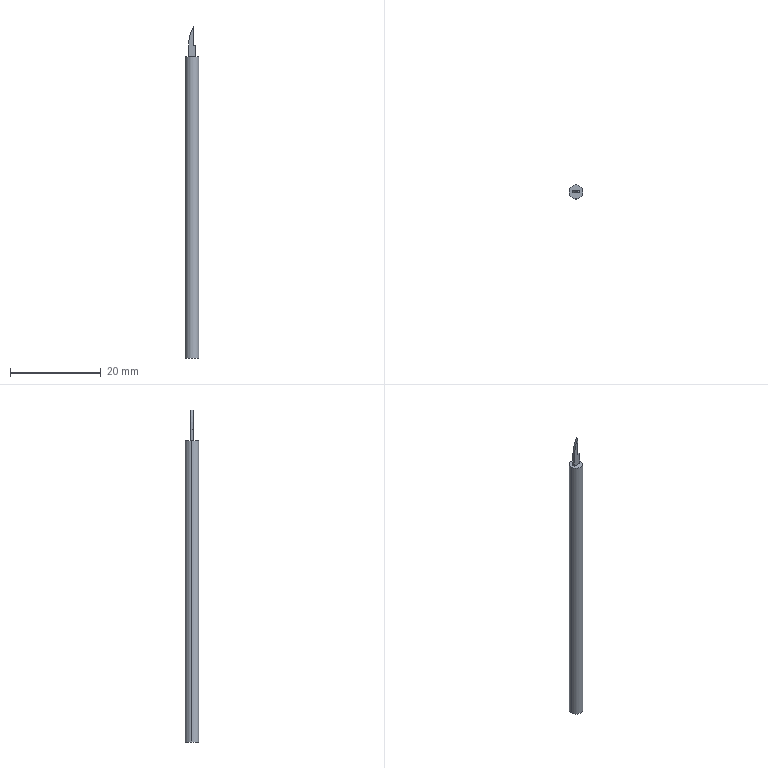Part | SolidWorks | features ICE 2, Extrusion 1 | 1 solid | 11 faces | box 3 x 3 x 73.338 mm | volume 473.804 mm3 | plane 8 | cylinder 3 | commonest cylinder face diameters 3 x2 16.855 x1
STEP:
#1=CARTESIAN_POINT('',(1.5,0.,-46.));
#2=VERTEX_POINT('',#1);
#3=CARTESIAN_POINT('',(-1.5,0.,-46.));
#4=VERTEX_POINT('',#3);
#5=CARTESIAN_POINT('',(0.,0.,-46.));
#6=DIRECTION('',(0.,0.,1.));
#7=DIRECTION('',(1.,0.,0.));
#8=AXIS2_PLACEMENT_3D('',#5,#6,#7);
#9=CIRCLE('',#8,1.5);
#10=EDGE_CURVE('',#2,#4,#9,.T.);
#11=ORIENTED_EDGE('',*,*,#10,.T.);
#12=CARTESIAN_POINT('',(-1.5,0.,20.5));
#13=VERTEX_POINT('',#12);
#14=CARTESIAN_POINT('',(-1.5,0.,-46.));
#15=DIRECTION('',(0.,0.,1.));
#16=VECTOR('',#15,1000.);
#17=LINE('',#14,#16);
#18=EDGE_CURVE('',#4,#13,#17,.T.);
#19=ORIENTED_EDGE('',*,*,#18,.T.);
#20=CARTESIAN_POINT('',(1.5,0.,20.5));
#21=VERTEX_POINT('',#20);
#22=CARTESIAN_POINT('',(0.,0.,20.5));
#23=DIRECTION('',(0.,0.,1.));
#24=DIRECTION('',(1.,0.,0.));
#25=AXIS2_PLACEMENT_3D('',#22,#23,#24);
#26=CIRCLE('',#25,1.5);
#27=EDGE_CURVE('',#21,#13,#26,.T.);
#28=ORIENTED_EDGE('',*,*,#27,.F.);
#29=CARTESIAN_POINT('',(1.5,0.,-46.));
#30=DIRECTION('',(0.,0.,1.));
#31=VECTOR('',#30,1000.);
#32=LINE('',#29,#31);
#33=EDGE_CURVE('',#2,#21,#32,.T.);
#34=ORIENTED_EDGE('',*,*,#33,.F.);
#35=EDGE_LOOP('',(#11,#19,#28,#34));
#36=FACE_OUTER_BOUND('',#35,.T.);
#37=CARTESIAN_POINT('',(0.,0.,-46.));
#38=DIRECTION('',(0.,0.,1.));
#39=DIRECTION('',(1.,0.,0.));
#40=AXIS2_PLACEMENT_3D('',#37,#38,#39);
#41=CYLINDRICAL_SURFACE('',#40,1.5);
#42=ADVANCED_FACE('',(#36),#41,.T.);
#43=ORIENTED_EDGE('',*,*,#27,.T.);
#44=CARTESIAN_POINT('',(0.,0.,20.5));
#45=DIRECTION('',(0.,0.,1.));
#46=DIRECTION('',(1.,0.,0.));
#47=AXIS2_PLACEMENT_3D('',#44,#45,#46);
#48=CIRCLE('',#47,1.5);
#49=EDGE_CURVE('',#13,#21,#48,.T.);
#50=ORIENTED_EDGE('',*,*,#49,.T.);
#51=EDGE_LOOP('',(#43,#50));
#52=FACE_OUTER_BOUND('',#51,.T.);
#53=CARTESIAN_POINT('',(0.8739,0.25,20.5));
#54=VERTEX_POINT('',#53);
#55=CARTESIAN_POINT('',(0.8739,-0.25,20.5));
#56=VERTEX_POINT('',#55);
#57=CARTESIAN_POINT('',(0.8739,0.25,20.5));
#58=DIRECTION('',(0.,-1.,0.));
#59=VECTOR('',#58,1000.);
#60=LINE('',#57,#59);
#61=EDGE_CURVE('',#54,#56,#60,.T.);
#62=ORIENTED_EDGE('',*,*,#61,.T.);
#63=CARTESIAN_POINT('',(-0.7579,-0.25,20.5));
#64=VERTEX_POINT('',#63);
#65=CARTESIAN_POINT('',(0.8739,-0.25,20.5));
#66=DIRECTION('',(-1.,0.,0.));
#67=VECTOR('',#66,1000.);
#68=LINE('',#65,#67);
#69=EDGE_CURVE('',#56,#64,#68,.T.);
#70=ORIENTED_EDGE('',*,*,#69,.T.);
#71=CARTESIAN_POINT('',(-0.7579,0.25,20.5));
#72=VERTEX_POINT('',#71);
#73=CARTESIAN_POINT('',(-0.7579,0.25,20.5));
#74=DIRECTION('',(0.,-1.,0.));
#75=VECTOR('',#74,1000.);
#76=LINE('',#73,#75);
#77=EDGE_CURVE('',#72,#64,#76,.T.);
#78=ORIENTED_EDGE('',*,*,#77,.F.);
#79=CARTESIAN_POINT('',(0.8739,0.25,20.5));
#80=DIRECTION('',(-1.,0.,0.));
#81=VECTOR('',#80,1000.);
#82=LINE('',#79,#81);
#83=EDGE_CURVE('',#54,#72,#82,.T.);
#84=ORIENTED_EDGE('',*,*,#83,.F.);
#85=EDGE_LOOP('',(#62,#70,#78,#84));
#86=FACE_BOUND('',#85,.T.);
#87=CARTESIAN_POINT('',(0.,0.,20.5));
#88=DIRECTION('',(0.,0.,1.));
#89=DIRECTION('',(1.,0.,0.));
#90=AXIS2_PLACEMENT_3D('',#87,#88,#89);
#91=PLANE('',#90);
#92=ADVANCED_FACE('',(#52,#86),#91,.T.);
#93=ORIENTED_EDGE('',*,*,#18,.F.);
#94=CARTESIAN_POINT('',(0.,0.,-46.));
#95=DIRECTION('',(0.,0.,1.));
#96=DIRECTION('',(1.,0.,0.));
#97=AXIS2_PLACEMENT_3D('',#94,#95,#96);
#98=CIRCLE('',#97,1.5);
#99=EDGE_CURVE('',#4,#2,#98,.T.);
#100=ORIENTED_EDGE('',*,*,#99,.T.);
#101=ORIENTED_EDGE('',*,*,#33,.T.);
#102=ORIENTED_EDGE('',*,*,#49,.F.);
#103=EDGE_LOOP('',(#93,#100,#101,#102));
#104=FACE_OUTER_BOUND('',#103,.T.);
#105=CARTESIAN_POINT('',(0.,0.,-46.));
#106=DIRECTION('',(0.,0.,1.));
#107=DIRECTION('',(1.,0.,0.));
#108=AXIS2_PLACEMENT_3D('',#105,#106,#107);
#109=CYLINDRICAL_SURFACE('',#108,1.5);
#110=ADVANCED_FACE('',(#104),#109,.T.);
#111=ORIENTED_EDGE('',*,*,#10,.F.);
#112=ORIENTED_EDGE('',*,*,#99,.F.);
#113=EDGE_LOOP('',(#111,#112));
#114=FACE_OUTER_BOUND('',#113,.T.);
#115=CARTESIAN_POINT('',(0.,0.,-46.));
#116=DIRECTION('',(0.,0.,1.));
#117=DIRECTION('',(1.,0.,0.));
#118=AXIS2_PLACEMENT_3D('',#115,#116,#117);
#119=PLANE('',#118);
#120=ADVANCED_FACE('',(#114),#119,.F.);
#121=CARTESIAN_POINT('',(0.8739,-0.25,23.139));
#122=VERTEX_POINT('',#121);
#123=CARTESIAN_POINT('',(0.8739,-0.25,23.139));
#124=DIRECTION('',(0.,0.,-1.));
#125=VECTOR('',#124,1000.);
#126=LINE('',#123,#125);
#127=EDGE_CURVE('',#122,#56,#126,.T.);
#128=ORIENTED_EDGE('',*,*,#127,.T.);
#129=ORIENTED_EDGE('',*,*,#61,.F.);
#130=CARTESIAN_POINT('',(0.8739,0.25,23.139));
#131=VERTEX_POINT('',#130);
#132=CARTESIAN_POINT('',(0.8739,0.25,23.139));
#133=DIRECTION('',(0.,0.,-1.));
#134=VECTOR('',#133,1000.);
#135=LINE('',#132,#134);
#136=EDGE_CURVE('',#131,#54,#135,.T.);
#137=ORIENTED_EDGE('',*,*,#136,.F.);
#138=CARTESIAN_POINT('',(0.8739,0.25,23.139));
#139=DIRECTION('',(0.,-1.,0.));
#140=VECTOR('',#139,1000.);
#141=LINE('',#138,#140);
#142=EDGE_CURVE('',#131,#122,#141,.T.);
#143=ORIENTED_EDGE('',*,*,#142,.T.);
#144=EDGE_LOOP('',(#128,#129,#137,#143));
#145=FACE_OUTER_BOUND('',#144,.T.);
#146=CARTESIAN_POINT('',(0.8739,0.25,23.139));
#147=DIRECTION('',(-1.,0.,0.));
#148=DIRECTION('',(0.,-1.,0.));
#149=AXIS2_PLACEMENT_3D('',#146,#147,#148);
#150=PLANE('',#149);
#151=ADVANCED_FACE('',(#145),#150,.F.);
#152=CARTESIAN_POINT('',(-0.7579,-0.25,23.139));
#153=VERTEX_POINT('',#152);
#154=CARTESIAN_POINT('',(-0.7579,-0.25,20.5));
#155=DIRECTION('',(0.,0.,1.));
#156=VECTOR('',#155,1000.);
#157=LINE('',#154,#156);
#158=EDGE_CURVE('',#64,#153,#157,.T.);
#159=ORIENTED_EDGE('',*,*,#158,.T.);
#160=CARTESIAN_POINT('',(-0.7579,0.25,23.139));
#161=VERTEX_POINT('',#160);
#162=CARTESIAN_POINT('',(-0.7579,0.25,23.139));
#163=DIRECTION('',(0.,-1.,0.));
#164=VECTOR('',#163,1000.);
#165=LINE('',#162,#164);
#166=EDGE_CURVE('',#161,#153,#165,.T.);
#167=ORIENTED_EDGE('',*,*,#166,.F.);
#168=CARTESIAN_POINT('',(-0.7579,0.25,20.5));
#169=DIRECTION('',(0.,0.,1.));
#170=VECTOR('',#169,1000.);
#171=LINE('',#168,#170);
#172=EDGE_CURVE('',#72,#161,#171,.T.);
#173=ORIENTED_EDGE('',*,*,#172,.F.);
#174=ORIENTED_EDGE('',*,*,#77,.T.);
#175=EDGE_LOOP('',(#159,#167,#173,#174));
#176=FACE_OUTER_BOUND('',#175,.T.);
#177=CARTESIAN_POINT('',(-0.7579,0.25,20.5));
#178=DIRECTION('',(1.,0.,0.));
#179=DIRECTION('',(0.,1.,0.));
#180=AXIS2_PLACEMENT_3D('',#177,#178,#179);
#181=PLANE('',#180);
#182=ADVANCED_FACE('',(#176),#181,.F.);
#183=CARTESIAN_POINT('',(0.3626,-0.25,27.338));
#184=VERTEX_POINT('',#183);
#185=CARTESIAN_POINT('',(7.67,-0.25,23.139));
#186=DIRECTION('',(0.,1.,0.));
#187=DIRECTION('',(0.,0.,1.));
#188=AXIS2_PLACEMENT_3D('',#185,#186,#187);
#189=CIRCLE('',#188,8.428);
#190=EDGE_CURVE('',#153,#184,#189,.T.);
#191=ORIENTED_EDGE('',*,*,#190,.T.);
#192=CARTESIAN_POINT('',(0.3626,0.25,27.338));
#193=VERTEX_POINT('',#192);
#194=CARTESIAN_POINT('',(0.3626,0.25,27.338));
#195=DIRECTION('',(0.,-1.,0.));
#196=VECTOR('',#195,1000.);
#197=LINE('',#194,#196);
#198=EDGE_CURVE('',#193,#184,#197,.T.);
#199=ORIENTED_EDGE('',*,*,#198,.F.);
#200=CARTESIAN_POINT('',(7.67,0.25,23.139));
#201=DIRECTION('',(0.,1.,0.));
#202=DIRECTION('',(0.,0.,1.));
#203=AXIS2_PLACEMENT_3D('',#200,#201,#202);
#204=CIRCLE('',#203,8.428);
#205=EDGE_CURVE('',#161,#193,#204,.T.);
#206=ORIENTED_EDGE('',*,*,#205,.F.);
#207=ORIENTED_EDGE('',*,*,#166,.T.);
#208=EDGE_LOOP('',(#191,#199,#206,#207));
#209=FACE_OUTER_BOUND('',#208,.T.);
#210=CARTESIAN_POINT('',(7.67,0.25,23.139));
#211=DIRECTION('',(0.,-1.,0.));
#212=DIRECTION('',(0.,0.,-1.));
#213=AXIS2_PLACEMENT_3D('',#210,#211,#212);
#214=CYLINDRICAL_SURFACE('',#213,8.428);
#215=ADVANCED_FACE('',(#209),#214,.T.);
#216=CARTESIAN_POINT('',(0.3626,-0.25,23.139));
#217=VERTEX_POINT('',#216);
#218=CARTESIAN_POINT('',(0.3626,-0.25,27.338));
#219=DIRECTION('',(0.,0.,-1.));
#220=VECTOR('',#219,1000.);
#221=LINE('',#218,#220);
#222=EDGE_CURVE('',#184,#217,#221,.T.);
#223=ORIENTED_EDGE('',*,*,#222,.T.);
#224=CARTESIAN_POINT('',(0.3626,0.25,23.139));
#225=VERTEX_POINT('',#224);
#226=CARTESIAN_POINT('',(0.3626,0.25,23.139));
#227=DIRECTION('',(0.,-1.,0.));
#228=VECTOR('',#227,1000.);
#229=LINE('',#226,#228);
#230=EDGE_CURVE('',#225,#217,#229,.T.);
#231=ORIENTED_EDGE('',*,*,#230,.F.);
#232=CARTESIAN_POINT('',(0.3626,0.25,27.338));
#233=DIRECTION('',(0.,0.,-1.));
#234=VECTOR('',#233,1000.);
#235=LINE('',#232,#234);
#236=EDGE_CURVE('',#193,#225,#235,.T.);
#237=ORIENTED_EDGE('',*,*,#236,.F.);
#238=ORIENTED_EDGE('',*,*,#198,.T.);
#239=EDGE_LOOP('',(#223,#231,#237,#238));
#240=FACE_OUTER_BOUND('',#239,.T.);
#241=CARTESIAN_POINT('',(0.3626,0.25,27.338));
#242=DIRECTION('',(-1.,0.,0.));
#243=DIRECTION('',(0.,-1.,0.));
#244=AXIS2_PLACEMENT_3D('',#241,#242,#243);
#245=PLANE('',#244);
#246=ADVANCED_FACE('',(#240),#245,.F.);
#247=CARTESIAN_POINT('',(0.3626,-0.25,23.139));
#248=DIRECTION('',(1.,0.,0.));
#249=VECTOR('',#248,1000.);
#250=LINE('',#247,#249);
#251=EDGE_CURVE('',#217,#122,#250,.T.);
#252=ORIENTED_EDGE('',*,*,#251,.T.);
#253=ORIENTED_EDGE('',*,*,#142,.F.);
#254=CARTESIAN_POINT('',(0.3626,0.25,23.139));
#255=DIRECTION('',(1.,0.,0.));
#256=VECTOR('',#255,1000.);
#257=LINE('',#254,#256);
#258=EDGE_CURVE('',#225,#131,#257,.T.);
#259=ORIENTED_EDGE('',*,*,#258,.F.);
#260=ORIENTED_EDGE('',*,*,#230,.T.);
#261=EDGE_LOOP('',(#252,#253,#259,#260));
#262=FACE_OUTER_BOUND('',#261,.T.);
#263=CARTESIAN_POINT('',(0.3626,0.25,23.139));
#264=DIRECTION('',(0.,0.,-1.));
#265=DIRECTION('',(0.,1.,0.));
#266=AXIS2_PLACEMENT_3D('',#263,#264,#265);
#267=PLANE('',#266);
#268=ADVANCED_FACE('',(#262),#267,.F.);
#269=ORIENTED_EDGE('',*,*,#136,.T.);
#270=ORIENTED_EDGE('',*,*,#83,.T.);
#271=ORIENTED_EDGE('',*,*,#172,.T.);
#272=ORIENTED_EDGE('',*,*,#205,.T.);
#273=ORIENTED_EDGE('',*,*,#236,.T.);
#274=ORIENTED_EDGE('',*,*,#258,.T.);
#275=EDGE_LOOP('',(#269,#270,#271,#272,#273,#274));
#276=FACE_OUTER_BOUND('',#275,.T.);
#277=CARTESIAN_POINT('',(7.67,0.25,23.139));
#278=DIRECTION('',(0.,1.,0.));
#279=DIRECTION('',(0.,0.,1.));
#280=AXIS2_PLACEMENT_3D('',#277,#278,#279);
#281=PLANE('',#280);
#282=ADVANCED_FACE('',(#276),#281,.T.);
#283=ORIENTED_EDGE('',*,*,#127,.F.);
#284=ORIENTED_EDGE('',*,*,#251,.F.);
#285=ORIENTED_EDGE('',*,*,#222,.F.);
#286=ORIENTED_EDGE('',*,*,#190,.F.);
#287=ORIENTED_EDGE('',*,*,#158,.F.);
#288=ORIENTED_EDGE('',*,*,#69,.F.);
#289=EDGE_LOOP('',(#283,#284,#285,#286,#287,#288));
#290=FACE_OUTER_BOUND('',#289,.T.);
#291=CARTESIAN_POINT('',(7.67,-0.25,23.139));
#292=DIRECTION('',(0.,1.,0.));
#293=DIRECTION('',(0.,0.,1.));
#294=AXIS2_PLACEMENT_3D('',#291,#292,#293);
#295=PLANE('',#294);
#296=ADVANCED_FACE('',(#290),#295,.F.);
#297=CLOSED_SHELL('',(#42,#92,#110,#120,#151,#182,#215,#246,#268,#282,#296));
#298=MANIFOLD_SOLID_BREP('',#297);
#299=CARTESIAN_POINT('',(0.,0.,0.));
#300=DIRECTION('',(0.,0.,1.));
#301=DIRECTION('',(1.,0.,0.));
#302=AXIS2_PLACEMENT_3D('',#299,#300,#301);
#303=(LENGTH_UNIT()NAMED_UNIT(*)SI_UNIT(.MILLI.,.METRE.));
#304=UNCERTAINTY_MEASURE_WITH_UNIT(LENGTH_MEASURE(0.00001),#303,'','');
#305=(NAMED_UNIT(*)PLANE_ANGLE_UNIT()SI_UNIT($,.RADIAN.));
#306=(NAMED_UNIT(*)SI_UNIT($,.STERADIAN.)SOLID_ANGLE_UNIT());
#307=(GEOMETRIC_REPRESENTATION_CONTEXT(3)GLOBAL_UNCERTAINTY_ASSIGNED_CONTEXT((#304))GLOBAL_UNIT_ASSIGNED_CONTEXT((#303,#305,#306))REPRESENTATION_CONTEXT('',''));
#308=ADVANCED_BREP_SHAPE_REPRESENTATION('',(#298,#302),#307);